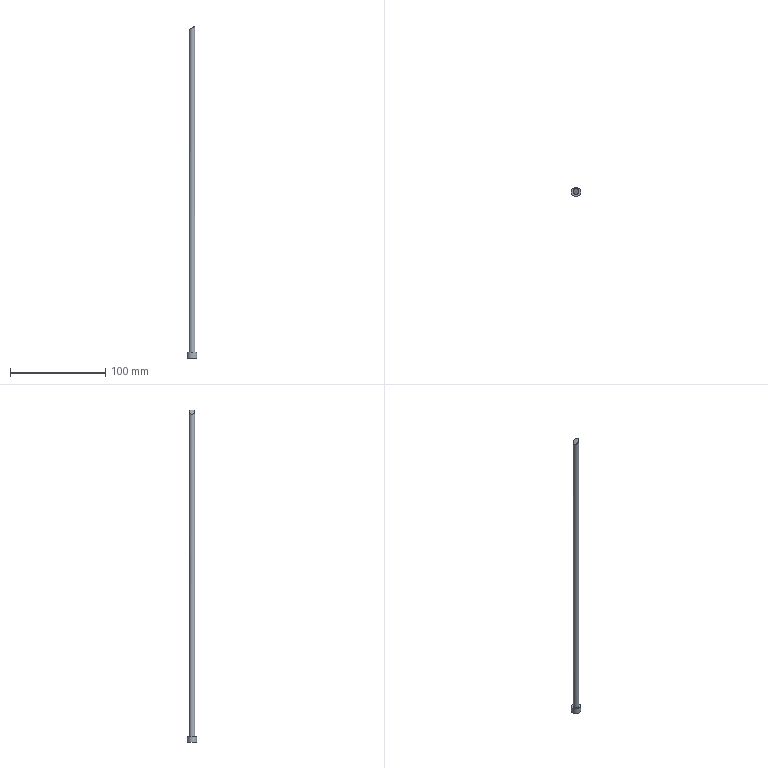Part | NX | features solid 2 | 1 solid | 5 faces | box 10 x 10 x 348.483 mm | volume 10095 mm3 | cylinder 2 | plane 2 | spline 1 | commonest cylinder face diameters 6 x1 10 x1
STEP:
#1=CARTESIAN_POINT('',(-26.5,69.,-339.5));
#2=VERTEX_POINT('',#1);
#3=CARTESIAN_POINT('',(-29.5,69.,-339.5));
#4=DIRECTION('',(0.,0.,1.));
#5=DIRECTION('',(1.,0.,0.));
#6=AXIS2_PLACEMENT_3D('',#3,#4,#5);
#7=CIRCLE('',#6,3.);
#8=EDGE_CURVE('',#2,#2,#7,.T.);
#9=ORIENTED_EDGE('',*,*,#8,.T.);
#10=EDGE_LOOP('',(#9));
#11=FACE_BOUND('',#10,.T.);
#12=CARTESIAN_POINT('',(-32.484,69.312,-1.395));
#13=VERTEX_POINT('',#12);
#14=CARTESIAN_POINT('',(-32.417,67.968,-1.301));
#15=CARTESIAN_POINT('',(-32.585,69.329,-1.477));
#16=CARTESIAN_POINT('',(-32.146,70.59,-1.165));
#17=CARTESIAN_POINT('',(-31.056,71.758,-0.3463));
#18=CARTESIAN_POINT('',(-29.256,72.242,0.9925));
#19=CARTESIAN_POINT('',(-27.487,71.47,2.252));
#20=CARTESIAN_POINT('',(-26.583,70.036,2.899));
#21=CARTESIAN_POINT('',(-26.415,68.686,3.046));
#22=CARTESIAN_POINT('',(-26.848,67.412,2.791));
#23=CARTESIAN_POINT('',(-27.982,66.208,2.052));
#24=CARTESIAN_POINT('',(-29.835,65.768,0.7512));
#25=CARTESIAN_POINT('',(-31.539,66.566,-0.5671));
#26=CARTESIAN_POINT('',(-32.417,67.968,-1.301));
#27=CARTESIAN_POINT('',(-32.585,69.329,-1.477));
#28=CARTESIAN_POINT('',(-32.146,70.59,-1.165));
#29=B_SPLINE_CURVE_WITH_KNOTS('',3,(#14,#15,#16,#17,#18,#19,#20,#21,#22,#23,#24,#25,#26,#27,#28),.UNSPECIFIED.,.T.,.F.,(1,1,1,1,1,1,1,1,1,1,1,1,1,1,1,1,1,1,1),(-0.005262,-0.002631,-0.001315,0.,0.001315,0.002631,0.005262,0.007893,0.009208,0.01052,0.01184,0.01315,0.01579,0.01842,0.01973,0.02105,0.02236,0.02368,0.02631),.UNSPECIFIED.);
#30=EDGE_CURVE('',#13,#13,#29,.T.);
#31=ORIENTED_EDGE('',*,*,#30,.T.);
#32=EDGE_LOOP('',(#31));
#33=FACE_BOUND('',#32,.T.);
#34=CARTESIAN_POINT('',(-29.5,69.,-345.5));
#35=DIRECTION('',(0.,0.,1.));
#36=DIRECTION('',(1.,0.,0.));
#37=AXIS2_PLACEMENT_3D('',#34,#35,#36);
#38=CYLINDRICAL_SURFACE('',#37,3.);
#39=ADVANCED_FACE('',(#11,#33),#38,.T.);
#40=ORIENTED_EDGE('',*,*,#8,.F.);
#41=EDGE_LOOP('',(#40));
#42=FACE_BOUND('',#41,.T.);
#43=CARTESIAN_POINT('',(-24.5,69.,-339.5));
#44=VERTEX_POINT('',#43);
#45=CARTESIAN_POINT('',(-29.5,69.,-339.5));
#46=DIRECTION('',(0.,0.,-1.));
#47=DIRECTION('',(1.,0.,0.));
#48=AXIS2_PLACEMENT_3D('',#45,#46,#47);
#49=CIRCLE('',#48,5.);
#50=EDGE_CURVE('',#44,#44,#49,.T.);
#51=ORIENTED_EDGE('',*,*,#50,.F.);
#52=EDGE_LOOP('',(#51));
#53=FACE_BOUND('',#52,.T.);
#54=CARTESIAN_POINT('',(-29.5,69.,-339.5));
#55=DIRECTION('',(0.,0.,1.));
#56=DIRECTION('',(1.,0.,0.));
#57=AXIS2_PLACEMENT_3D('',#54,#55,#56);
#58=PLANE('',#57);
#59=ADVANCED_FACE('',(#42,#53),#58,.T.);
#60=CARTESIAN_POINT('',(-24.5,69.,-345.5));
#61=VERTEX_POINT('',#60);
#62=CARTESIAN_POINT('',(-29.5,69.,-345.5));
#63=DIRECTION('',(0.,0.,1.));
#64=DIRECTION('',(1.,0.,0.));
#65=AXIS2_PLACEMENT_3D('',#62,#63,#64);
#66=CIRCLE('',#65,5.);
#67=EDGE_CURVE('',#61,#61,#66,.T.);
#68=ORIENTED_EDGE('',*,*,#67,.F.);
#69=EDGE_LOOP('',(#68));
#70=FACE_BOUND('',#69,.T.);
#71=CARTESIAN_POINT('',(-29.5,69.,-345.5));
#72=DIRECTION('',(0.,0.,-1.));
#73=DIRECTION('',(-1.,0.,0.));
#74=AXIS2_PLACEMENT_3D('',#71,#72,#73);
#75=PLANE('',#74);
#76=ADVANCED_FACE('',(#70),#75,.T.);
#77=ORIENTED_EDGE('',*,*,#50,.T.);
#78=EDGE_LOOP('',(#77));
#79=FACE_BOUND('',#78,.T.);
#80=ORIENTED_EDGE('',*,*,#67,.T.);
#81=EDGE_LOOP('',(#80));
#82=FACE_BOUND('',#81,.T.);
#83=CARTESIAN_POINT('',(-29.5,69.,-345.5));
#84=DIRECTION('',(0.,0.,1.));
#85=DIRECTION('',(1.,0.,0.));
#86=AXIS2_PLACEMENT_3D('',#83,#84,#85);
#87=CYLINDRICAL_SURFACE('',#86,5.);
#88=ADVANCED_FACE('',(#79,#82),#87,.T.);
#89=ORIENTED_EDGE('',*,*,#30,.F.);
#90=EDGE_LOOP('',(#89));
#91=FACE_BOUND('',#90,.T.);
#92=CARTESIAN_POINT('',(-32.582,65.94,-1.372));
#93=CARTESIAN_POINT('',(-32.559,67.98,-1.416));
#94=CARTESIAN_POINT('',(-32.536,70.019,-1.458));
#95=CARTESIAN_POINT('',(-32.512,72.059,-1.5));
#96=CARTESIAN_POINT('',(-30.615,65.94,0.1934));
#97=CARTESIAN_POINT('',(-30.593,67.98,0.1506));
#98=CARTESIAN_POINT('',(-30.571,70.02,0.1087));
#99=CARTESIAN_POINT('',(-30.548,72.06,0.06804));
#100=CARTESIAN_POINT('',(-28.58,65.941,1.675));
#101=CARTESIAN_POINT('',(-28.56,67.981,1.634));
#102=CARTESIAN_POINT('',(-28.539,70.02,1.593));
#103=CARTESIAN_POINT('',(-28.517,72.06,1.553));
#104=CARTESIAN_POINT('',(-26.487,65.941,3.071));
#105=CARTESIAN_POINT('',(-26.467,67.981,3.03));
#106=CARTESIAN_POINT('',(-26.447,70.021,2.99));
#107=CARTESIAN_POINT('',(-26.426,72.06,2.952));
#108=B_SPLINE_SURFACE_WITH_KNOTS('',3,3,((#92,#93,#94,#95),(#96,#97,#98,#99),(#100,#101,#102,#103),(#104,#105,#106,#107)),.UNSPECIFIED.,.F.,.F.,.F.,(4,4),(4,4),(0.4584,0.4967),(0.8038,0.92),.PIECEWISE_BEZIER_KNOTS.);
#109=ADVANCED_FACE('',(#91),#108,.T.);
#110=CLOSED_SHELL('',(#39,#59,#76,#88,#109));
#111=MANIFOLD_SOLID_BREP('',#110);
#112=(LENGTH_UNIT()NAMED_UNIT(*)SI_UNIT(.MILLI.,.METRE.));
#113=UNCERTAINTY_MEASURE_WITH_UNIT(LENGTH_MEASURE(0.0508),#112,'','');
#114=(NAMED_UNIT(*)PLANE_ANGLE_UNIT()SI_UNIT($,.RADIAN.));
#115=(NAMED_UNIT(*)SI_UNIT($,.STERADIAN.)SOLID_ANGLE_UNIT());
#116=(GEOMETRIC_REPRESENTATION_CONTEXT(3)GLOBAL_UNCERTAINTY_ASSIGNED_CONTEXT((#113))GLOBAL_UNIT_ASSIGNED_CONTEXT((#112,#114,#115))REPRESENTATION_CONTEXT('',''));
#117=ADVANCED_BREP_SHAPE_REPRESENTATION('',(#111),#116);